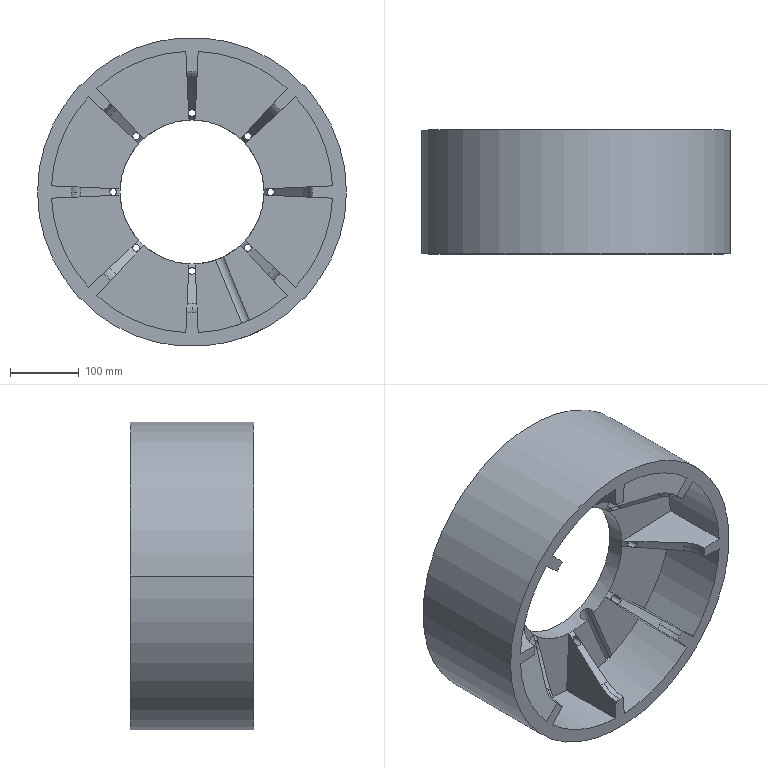Part | SolidWorks | features ICE 3, Revolution 2, CirPattern 1 | 1 solid | 132 faces | box 450 x 180.45 x 450 mm | volume 8519490 mm3 | plane 52 | cylinder 40 | cone 24 | torus 16 | commonest cylinder face diameters 10 x16 410 x16 20 x2 210 x2 280 x2 450 x2